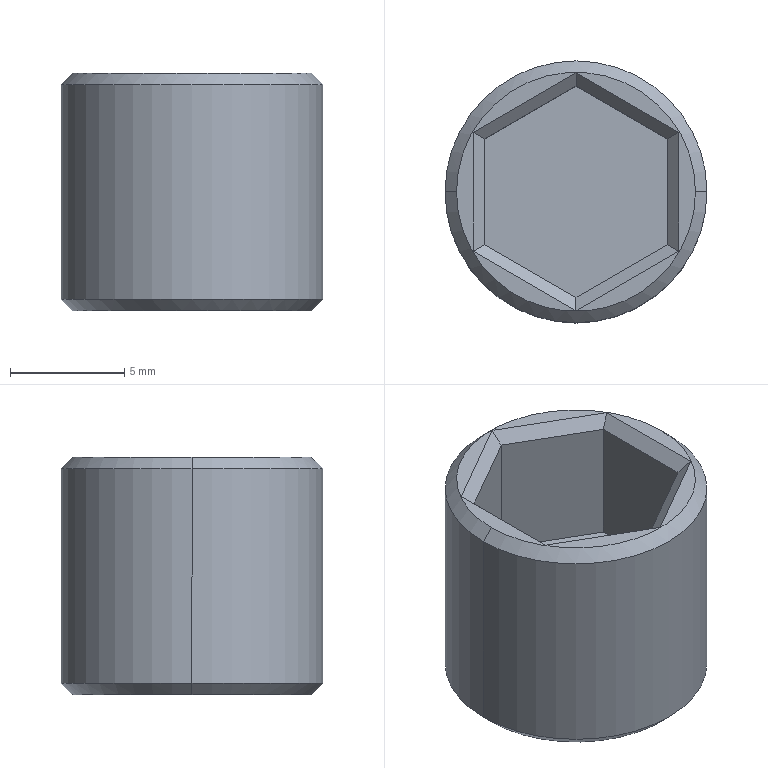Part | SolidWorks | features BaseBody 1 | 1 solid | 21 faces | box 11.45 x 11.45 x 10.4 mm | volume 725.97 mm3 | plane 15 | cone 4 | cylinder 2 | commonest cylinder face diameters 11.45 x2
STEP:
#1=CARTESIAN_POINT('',(5.725,0.,0.5));
#2=VERTEX_POINT('',#1);
#3=CARTESIAN_POINT('',(-5.725,0.,0.5));
#4=VERTEX_POINT('',#3);
#5=CARTESIAN_POINT('',(0.,0.,0.5));
#6=DIRECTION('',(0.,0.,1.));
#7=DIRECTION('',(1.,0.,0.));
#8=AXIS2_PLACEMENT_3D('',#5,#6,#7);
#9=CIRCLE('',#8,5.725);
#10=EDGE_CURVE('',#2,#4,#9,.T.);
#11=ORIENTED_EDGE('',*,*,#10,.T.);
#12=CARTESIAN_POINT('',(-5.725,0.,9.9));
#13=VERTEX_POINT('',#12);
#14=CARTESIAN_POINT('',(-5.725,0.,0.));
#15=DIRECTION('',(0.,0.,1.));
#16=VECTOR('',#15,1000.);
#17=LINE('',#14,#16);
#18=EDGE_CURVE('',#4,#13,#17,.T.);
#19=ORIENTED_EDGE('',*,*,#18,.T.);
#20=CARTESIAN_POINT('',(5.725,0.,9.9));
#21=VERTEX_POINT('',#20);
#22=CARTESIAN_POINT('',(0.,0.,9.9));
#23=DIRECTION('',(0.,0.,-1.));
#24=DIRECTION('',(1.,0.,0.));
#25=AXIS2_PLACEMENT_3D('',#22,#23,#24);
#26=CIRCLE('',#25,5.725);
#27=EDGE_CURVE('',#13,#21,#26,.T.);
#28=ORIENTED_EDGE('',*,*,#27,.T.);
#29=CARTESIAN_POINT('',(5.725,0.,0.));
#30=DIRECTION('',(0.,0.,1.));
#31=VECTOR('',#30,1000.);
#32=LINE('',#29,#31);
#33=EDGE_CURVE('',#2,#21,#32,.T.);
#34=ORIENTED_EDGE('',*,*,#33,.F.);
#35=EDGE_LOOP('',(#11,#19,#28,#34));
#36=FACE_OUTER_BOUND('',#35,.T.);
#37=CARTESIAN_POINT('',(0.,0.,0.));
#38=DIRECTION('',(0.,0.,1.));
#39=DIRECTION('',(1.,0.,0.));
#40=AXIS2_PLACEMENT_3D('',#37,#38,#39);
#41=CYLINDRICAL_SURFACE('',#40,5.725);
#42=ADVANCED_FACE('',(#36),#41,.T.);
#43=CARTESIAN_POINT('',(-5.225,0.,10.4));
#44=VERTEX_POINT('',#43);
#45=CARTESIAN_POINT('',(5.225,0.,10.4));
#46=VERTEX_POINT('',#45);
#47=CARTESIAN_POINT('',(0.,0.,10.4));
#48=DIRECTION('',(0.,0.,-1.));
#49=DIRECTION('',(-1.,0.,0.));
#50=AXIS2_PLACEMENT_3D('',#47,#48,#49);
#51=CIRCLE('',#50,5.225);
#52=EDGE_CURVE('',#44,#46,#51,.T.);
#53=ORIENTED_EDGE('',*,*,#52,.T.);
#54=CARTESIAN_POINT('',(5.725,0.,9.9));
#55=DIRECTION('',(0.7071,0.,-0.7071));
#56=VECTOR('',#55,1000.);
#57=LINE('',#54,#56);
#58=EDGE_CURVE('',#46,#21,#57,.T.);
#59=ORIENTED_EDGE('',*,*,#58,.T.);
#60=ORIENTED_EDGE('',*,*,#27,.F.);
#61=CARTESIAN_POINT('',(-5.725,0.,9.9));
#62=DIRECTION('',(-0.7071,0.,-0.7071));
#63=VECTOR('',#62,1000.);
#64=LINE('',#61,#63);
#65=EDGE_CURVE('',#44,#13,#64,.T.);
#66=ORIENTED_EDGE('',*,*,#65,.F.);
#67=EDGE_LOOP('',(#53,#59,#60,#66));
#68=FACE_OUTER_BOUND('',#67,.T.);
#69=CARTESIAN_POINT('',(0.,0.,9.9));
#70=DIRECTION('',(0.,0.,-1.));
#71=DIRECTION('',(-1.,0.,0.));
#72=AXIS2_PLACEMENT_3D('',#69,#70,#71);
#73=CONICAL_SURFACE('',#72,5.725,0.7854);
#74=ADVANCED_FACE('',(#68),#73,.T.);
#75=CARTESIAN_POINT('',(5.225,0.,0.));
#76=VERTEX_POINT('',#75);
#77=CARTESIAN_POINT('',(-5.225,0.,0.));
#78=VERTEX_POINT('',#77);
#79=CARTESIAN_POINT('',(0.,0.,0.));
#80=DIRECTION('',(0.,0.,1.));
#81=DIRECTION('',(1.,0.,0.));
#82=AXIS2_PLACEMENT_3D('',#79,#80,#81);
#83=CIRCLE('',#82,5.225);
#84=EDGE_CURVE('',#76,#78,#83,.T.);
#85=ORIENTED_EDGE('',*,*,#84,.T.);
#86=CARTESIAN_POINT('',(-5.725,0.,0.5));
#87=DIRECTION('',(-0.7071,0.,0.7071));
#88=VECTOR('',#87,1000.);
#89=LINE('',#86,#88);
#90=EDGE_CURVE('',#78,#4,#89,.T.);
#91=ORIENTED_EDGE('',*,*,#90,.T.);
#92=ORIENTED_EDGE('',*,*,#10,.F.);
#93=CARTESIAN_POINT('',(5.725,0.,0.5));
#94=DIRECTION('',(0.7071,0.,0.7071));
#95=VECTOR('',#94,1000.);
#96=LINE('',#93,#95);
#97=EDGE_CURVE('',#76,#2,#96,.T.);
#98=ORIENTED_EDGE('',*,*,#97,.F.);
#99=EDGE_LOOP('',(#85,#91,#92,#98));
#100=FACE_OUTER_BOUND('',#99,.T.);
#101=CARTESIAN_POINT('',(0.,0.,0.5));
#102=DIRECTION('',(0.,0.,1.));
#103=DIRECTION('',(1.,0.,0.));
#104=AXIS2_PLACEMENT_3D('',#101,#102,#103);
#105=CONICAL_SURFACE('',#104,5.725,0.7854);
#106=ADVANCED_FACE('',(#100),#105,.T.);
#107=ORIENTED_EDGE('',*,*,#18,.F.);
#108=CARTESIAN_POINT('',(0.,0.,0.5));
#109=DIRECTION('',(0.,0.,1.));
#110=DIRECTION('',(1.,0.,0.));
#111=AXIS2_PLACEMENT_3D('',#108,#109,#110);
#112=CIRCLE('',#111,5.725);
#113=EDGE_CURVE('',#4,#2,#112,.T.);
#114=ORIENTED_EDGE('',*,*,#113,.T.);
#115=ORIENTED_EDGE('',*,*,#33,.T.);
#116=CARTESIAN_POINT('',(0.,0.,9.9));
#117=DIRECTION('',(0.,0.,-1.));
#118=DIRECTION('',(1.,0.,0.));
#119=AXIS2_PLACEMENT_3D('',#116,#117,#118);
#120=CIRCLE('',#119,5.725);
#121=EDGE_CURVE('',#21,#13,#120,.T.);
#122=ORIENTED_EDGE('',*,*,#121,.T.);
#123=EDGE_LOOP('',(#107,#114,#115,#122));
#124=FACE_OUTER_BOUND('',#123,.T.);
#125=CARTESIAN_POINT('',(0.,0.,0.));
#126=DIRECTION('',(0.,0.,1.));
#127=DIRECTION('',(1.,0.,0.));
#128=AXIS2_PLACEMENT_3D('',#125,#126,#127);
#129=CYLINDRICAL_SURFACE('',#128,5.725);
#130=ADVANCED_FACE('',(#124),#129,.T.);
#131=ORIENTED_EDGE('',*,*,#58,.F.);
#132=CARTESIAN_POINT('',(0.,0.,10.4));
#133=DIRECTION('',(0.,0.,-1.));
#134=DIRECTION('',(-1.,0.,0.));
#135=AXIS2_PLACEMENT_3D('',#132,#133,#134);
#136=CIRCLE('',#135,5.225);
#137=EDGE_CURVE('',#46,#44,#136,.T.);
#138=ORIENTED_EDGE('',*,*,#137,.T.);
#139=ORIENTED_EDGE('',*,*,#65,.T.);
#140=ORIENTED_EDGE('',*,*,#121,.F.);
#141=EDGE_LOOP('',(#131,#138,#139,#140));
#142=FACE_OUTER_BOUND('',#141,.T.);
#143=CARTESIAN_POINT('',(0.,0.,9.9));
#144=DIRECTION('',(0.,0.,-1.));
#145=DIRECTION('',(-1.,0.,0.));
#146=AXIS2_PLACEMENT_3D('',#143,#144,#145);
#147=CONICAL_SURFACE('',#146,5.725,0.7854);
#148=ADVANCED_FACE('',(#142),#147,.T.);
#149=ORIENTED_EDGE('',*,*,#90,.F.);
#150=CARTESIAN_POINT('',(0.,0.,0.));
#151=DIRECTION('',(0.,0.,1.));
#152=DIRECTION('',(1.,0.,0.));
#153=AXIS2_PLACEMENT_3D('',#150,#151,#152);
#154=CIRCLE('',#153,5.225);
#155=EDGE_CURVE('',#78,#76,#154,.T.);
#156=ORIENTED_EDGE('',*,*,#155,.T.);
#157=ORIENTED_EDGE('',*,*,#97,.T.);
#158=ORIENTED_EDGE('',*,*,#113,.F.);
#159=EDGE_LOOP('',(#149,#156,#157,#158));
#160=FACE_OUTER_BOUND('',#159,.T.);
#161=CARTESIAN_POINT('',(0.,0.,0.5));
#162=DIRECTION('',(0.,0.,1.));
#163=DIRECTION('',(1.,0.,0.));
#164=AXIS2_PLACEMENT_3D('',#161,#162,#163);
#165=CONICAL_SURFACE('',#164,5.725,0.7854);
#166=ADVANCED_FACE('',(#160),#165,.T.);
#167=CARTESIAN_POINT('',(4.5,-2.598,10.4));
#168=VERTEX_POINT('',#167);
#169=CARTESIAN_POINT('',(4.5,2.598,10.4));
#170=VERTEX_POINT('',#169);
#171=CARTESIAN_POINT('',(4.5,0.,10.4));
#172=DIRECTION('',(0.,1.,0.));
#173=VECTOR('',#172,1000.);
#174=LINE('',#171,#173);
#175=EDGE_CURVE('',#168,#170,#174,.T.);
#176=ORIENTED_EDGE('',*,*,#175,.F.);
#177=CARTESIAN_POINT('',(0.,-5.196,10.4));
#178=VERTEX_POINT('',#177);
#179=CARTESIAN_POINT('',(0.,-5.196,10.4));
#180=DIRECTION('',(0.866,0.5,0.));
#181=VECTOR('',#180,1000.);
#182=LINE('',#179,#181);
#183=EDGE_CURVE('',#178,#168,#182,.T.);
#184=ORIENTED_EDGE('',*,*,#183,.F.);
#185=CARTESIAN_POINT('',(-4.5,-2.598,10.4));
#186=VERTEX_POINT('',#185);
#187=CARTESIAN_POINT('',(-4.5,-2.598,10.4));
#188=DIRECTION('',(0.866,-0.5,0.));
#189=VECTOR('',#188,1000.);
#190=LINE('',#187,#189);
#191=EDGE_CURVE('',#186,#178,#190,.T.);
#192=ORIENTED_EDGE('',*,*,#191,.F.);
#193=CARTESIAN_POINT('',(-4.5,2.598,10.4));
#194=VERTEX_POINT('',#193);
#195=CARTESIAN_POINT('',(-4.5,0.,10.4));
#196=DIRECTION('',(0.,-1.,0.));
#197=VECTOR('',#196,1000.);
#198=LINE('',#195,#197);
#199=EDGE_CURVE('',#194,#186,#198,.T.);
#200=ORIENTED_EDGE('',*,*,#199,.F.);
#201=CARTESIAN_POINT('',(0.,5.196,10.4));
#202=VERTEX_POINT('',#201);
#203=CARTESIAN_POINT('',(0.,5.196,10.4));
#204=DIRECTION('',(-0.866,-0.5,0.));
#205=VECTOR('',#204,1000.);
#206=LINE('',#203,#205);
#207=EDGE_CURVE('',#202,#194,#206,.T.);
#208=ORIENTED_EDGE('',*,*,#207,.F.);
#209=CARTESIAN_POINT('',(4.5,2.598,10.4));
#210=DIRECTION('',(-0.866,0.5,0.));
#211=VECTOR('',#210,1000.);
#212=LINE('',#209,#211);
#213=EDGE_CURVE('',#170,#202,#212,.T.);
#214=ORIENTED_EDGE('',*,*,#213,.F.);
#215=EDGE_LOOP('',(#176,#184,#192,#200,#208,#214));
#216=FACE_BOUND('',#215,.T.);
#217=ORIENTED_EDGE('',*,*,#52,.F.);
#218=ORIENTED_EDGE('',*,*,#137,.F.);
#219=EDGE_LOOP('',(#217,#218));
#220=FACE_OUTER_BOUND('',#219,.T.);
#221=CARTESIAN_POINT('',(0.,0.,10.4));
#222=DIRECTION('',(0.,0.,-1.));
#223=DIRECTION('',(-1.,0.,0.));
#224=AXIS2_PLACEMENT_3D('',#221,#222,#223);
#225=PLANE('',#224);
#226=ADVANCED_FACE('',(#216,#220),#225,.F.);
#227=ORIENTED_EDGE('',*,*,#84,.F.);
#228=ORIENTED_EDGE('',*,*,#155,.F.);
#229=EDGE_LOOP('',(#227,#228));
#230=FACE_OUTER_BOUND('',#229,.T.);
#231=CARTESIAN_POINT('',(0.,0.,0.));
#232=DIRECTION('',(0.,0.,-1.));
#233=DIRECTION('',(-1.,0.,0.));
#234=AXIS2_PLACEMENT_3D('',#231,#232,#233);
#235=PLANE('',#234);
#236=ADVANCED_FACE('',(#230),#235,.T.);
#237=CARTESIAN_POINT('',(0.,4.619,9.9));
#238=VERTEX_POINT('',#237);
#239=CARTESIAN_POINT('',(0.,3.876,9.257));
#240=DIRECTION('',(0.,-0.7559,-0.6547));
#241=VECTOR('',#240,1000.);
#242=LINE('',#239,#241);
#243=EDGE_CURVE('',#202,#238,#242,.T.);
#244=ORIENTED_EDGE('',*,*,#243,.T.);
#245=CARTESIAN_POINT('',(4.,2.309,9.9));
#246=VERTEX_POINT('',#245);
#247=CARTESIAN_POINT('',(0.,4.619,9.9));
#248=DIRECTION('',(0.866,-0.5,0.));
#249=VECTOR('',#248,1000.);
#250=LINE('',#247,#249);
#251=EDGE_CURVE('',#238,#246,#250,.T.);
#252=ORIENTED_EDGE('',*,*,#251,.T.);
#253=CARTESIAN_POINT('',(4.,2.309,9.9));
#254=DIRECTION('',(0.6547,0.378,0.6547));
#255=VECTOR('',#254,1000.);
#256=LINE('',#253,#255);
#257=EDGE_CURVE('',#246,#170,#256,.T.);
#258=ORIENTED_EDGE('',*,*,#257,.T.);
#259=ORIENTED_EDGE('',*,*,#213,.T.);
#260=EDGE_LOOP('',(#244,#252,#258,#259));
#261=FACE_OUTER_BOUND('',#260,.T.);
#262=CARTESIAN_POINT('',(3.125,3.103,10.15));
#263=DIRECTION('',(-0.3536,-0.6124,0.7071));
#264=DIRECTION('',(0.,-0.7559,-0.6547));
#265=AXIS2_PLACEMENT_3D('',#262,#263,#264);
#266=PLANE('',#265);
#267=ADVANCED_FACE('',(#261),#266,.T.);
#268=ORIENTED_EDGE('',*,*,#257,.F.);
#269=CARTESIAN_POINT('',(4.,-2.309,9.9));
#270=VERTEX_POINT('',#269);
#271=CARTESIAN_POINT('',(4.,-1.155,9.9));
#272=DIRECTION('',(0.,-1.,0.));
#273=VECTOR('',#272,1000.);
#274=LINE('',#271,#273);
#275=EDGE_CURVE('',#246,#270,#274,.T.);
#276=ORIENTED_EDGE('',*,*,#275,.T.);
#277=CARTESIAN_POINT('',(4.,-2.309,9.9));
#278=DIRECTION('',(0.6547,-0.378,0.6547));
#279=VECTOR('',#278,1000.);
#280=LINE('',#277,#279);
#281=EDGE_CURVE('',#270,#168,#280,.T.);
#282=ORIENTED_EDGE('',*,*,#281,.T.);
#283=ORIENTED_EDGE('',*,*,#175,.T.);
#284=EDGE_LOOP('',(#268,#276,#282,#283));
#285=FACE_OUTER_BOUND('',#284,.T.);
#286=CARTESIAN_POINT('',(4.25,-1.155,10.15));
#287=DIRECTION('',(-0.7071,0.,0.7071));
#288=DIRECTION('',(0.7071,0.,0.7071));
#289=AXIS2_PLACEMENT_3D('',#286,#287,#288);
#290=PLANE('',#289);
#291=ADVANCED_FACE('',(#285),#290,.T.);
#292=ORIENTED_EDGE('',*,*,#281,.F.);
#293=CARTESIAN_POINT('',(0.,-4.619,9.9));
#294=VERTEX_POINT('',#293);
#295=CARTESIAN_POINT('',(4.,-2.309,9.9));
#296=DIRECTION('',(-0.866,-0.5,0.));
#297=VECTOR('',#296,1000.);
#298=LINE('',#295,#297);
#299=EDGE_CURVE('',#270,#294,#298,.T.);
#300=ORIENTED_EDGE('',*,*,#299,.T.);
#301=CARTESIAN_POINT('',(0.,-4.536,9.829));
#302=DIRECTION('',(0.,-0.7559,0.6547));
#303=VECTOR('',#302,1000.);
#304=LINE('',#301,#303);
#305=EDGE_CURVE('',#294,#178,#304,.T.);
#306=ORIENTED_EDGE('',*,*,#305,.T.);
#307=ORIENTED_EDGE('',*,*,#183,.T.);
#308=EDGE_LOOP('',(#292,#300,#306,#307));
#309=FACE_OUTER_BOUND('',#308,.T.);
#310=CARTESIAN_POINT('',(1.125,-4.258,10.15));
#311=DIRECTION('',(-0.3536,0.6124,0.7071));
#312=DIRECTION('',(0.,-0.7559,0.6547));
#313=AXIS2_PLACEMENT_3D('',#310,#311,#312);
#314=PLANE('',#313);
#315=ADVANCED_FACE('',(#309),#314,.T.);
#316=ORIENTED_EDGE('',*,*,#305,.F.);
#317=CARTESIAN_POINT('',(-4.,-2.309,9.9));
#318=VERTEX_POINT('',#317);
#319=CARTESIAN_POINT('',(0.,-4.619,9.9));
#320=DIRECTION('',(-0.866,0.5,0.));
#321=VECTOR('',#320,1000.);
#322=LINE('',#319,#321);
#323=EDGE_CURVE('',#294,#318,#322,.T.);
#324=ORIENTED_EDGE('',*,*,#323,.T.);
#325=CARTESIAN_POINT('',(-4.,-2.309,9.9));
#326=DIRECTION('',(-0.6547,-0.378,0.6547));
#327=VECTOR('',#326,1000.);
#328=LINE('',#325,#327);
#329=EDGE_CURVE('',#318,#186,#328,.T.);
#330=ORIENTED_EDGE('',*,*,#329,.T.);
#331=ORIENTED_EDGE('',*,*,#191,.T.);
#332=EDGE_LOOP('',(#316,#324,#330,#331));
#333=FACE_OUTER_BOUND('',#332,.T.);
#334=CARTESIAN_POINT('',(-3.125,-3.103,10.15));
#335=DIRECTION('',(0.3536,0.6124,0.7071));
#336=DIRECTION('',(0.,-0.7559,0.6547));
#337=AXIS2_PLACEMENT_3D('',#334,#335,#336);
#338=PLANE('',#337);
#339=ADVANCED_FACE('',(#333),#338,.T.);
#340=ORIENTED_EDGE('',*,*,#329,.F.);
#341=CARTESIAN_POINT('',(-4.,2.309,9.9));
#342=VERTEX_POINT('',#341);
#343=CARTESIAN_POINT('',(-4.,1.155,9.9));
#344=DIRECTION('',(0.,1.,0.));
#345=VECTOR('',#344,1000.);
#346=LINE('',#343,#345);
#347=EDGE_CURVE('',#318,#342,#346,.T.);
#348=ORIENTED_EDGE('',*,*,#347,.T.);
#349=CARTESIAN_POINT('',(-4.,2.309,9.9));
#350=DIRECTION('',(-0.6547,0.378,0.6547));
#351=VECTOR('',#350,1000.);
#352=LINE('',#349,#351);
#353=EDGE_CURVE('',#342,#194,#352,.T.);
#354=ORIENTED_EDGE('',*,*,#353,.T.);
#355=ORIENTED_EDGE('',*,*,#199,.T.);
#356=EDGE_LOOP('',(#340,#348,#354,#355));
#357=FACE_OUTER_BOUND('',#356,.T.);
#358=CARTESIAN_POINT('',(-4.25,1.155,10.15));
#359=DIRECTION('',(0.7071,0.,0.7071));
#360=DIRECTION('',(0.7071,0.,-0.7071));
#361=AXIS2_PLACEMENT_3D('',#358,#359,#360);
#362=PLANE('',#361);
#363=ADVANCED_FACE('',(#357),#362,.T.);
#364=ORIENTED_EDGE('',*,*,#353,.F.);
#365=CARTESIAN_POINT('',(-4.,2.309,9.9));
#366=DIRECTION('',(0.866,0.5,0.));
#367=VECTOR('',#366,1000.);
#368=LINE('',#365,#367);
#369=EDGE_CURVE('',#342,#238,#368,.T.);
#370=ORIENTED_EDGE('',*,*,#369,.T.);
#371=ORIENTED_EDGE('',*,*,#243,.F.);
#372=ORIENTED_EDGE('',*,*,#207,.T.);
#373=EDGE_LOOP('',(#364,#370,#371,#372));
#374=FACE_OUTER_BOUND('',#373,.T.);
#375=CARTESIAN_POINT('',(-1.125,4.258,10.15));
#376=DIRECTION('',(0.3536,-0.6124,0.7071));
#377=DIRECTION('',(0.,-0.7559,-0.6547));
#378=AXIS2_PLACEMENT_3D('',#375,#376,#377);
#379=PLANE('',#378);
#380=ADVANCED_FACE('',(#374),#379,.T.);
#381=CARTESIAN_POINT('',(4.,2.309,4.4));
#382=VERTEX_POINT('',#381);
#383=CARTESIAN_POINT('',(0.,4.619,4.4));
#384=VERTEX_POINT('',#383);
#385=CARTESIAN_POINT('',(4.,2.309,4.4));
#386=DIRECTION('',(-0.866,0.5,0.));
#387=VECTOR('',#386,1000.);
#388=LINE('',#385,#387);
#389=EDGE_CURVE('',#382,#384,#388,.T.);
#390=ORIENTED_EDGE('',*,*,#389,.F.);
#391=CARTESIAN_POINT('',(4.,2.309,10.4));
#392=DIRECTION('',(0.,0.,-1.));
#393=VECTOR('',#392,1000.);
#394=LINE('',#391,#393);
#395=EDGE_CURVE('',#246,#382,#394,.T.);
#396=ORIENTED_EDGE('',*,*,#395,.F.);
#397=ORIENTED_EDGE('',*,*,#251,.F.);
#398=CARTESIAN_POINT('',(0.,4.619,10.4));
#399=DIRECTION('',(0.,0.,1.));
#400=VECTOR('',#399,1000.);
#401=LINE('',#398,#400);
#402=EDGE_CURVE('',#384,#238,#401,.T.);
#403=ORIENTED_EDGE('',*,*,#402,.F.);
#404=EDGE_LOOP('',(#390,#396,#397,#403));
#405=FACE_OUTER_BOUND('',#404,.T.);
#406=CARTESIAN_POINT('',(4.,2.309,10.4));
#407=DIRECTION('',(0.5,0.866,0.));
#408=DIRECTION('',(-0.866,0.5,0.));
#409=AXIS2_PLACEMENT_3D('',#406,#407,#408);
#410=PLANE('',#409);
#411=ADVANCED_FACE('',(#405),#410,.F.);
#412=CARTESIAN_POINT('',(4.,-2.309,4.4));
#413=VERTEX_POINT('',#412);
#414=CARTESIAN_POINT('',(4.,-2.309,4.4));
#415=DIRECTION('',(0.,1.,0.));
#416=VECTOR('',#415,1000.);
#417=LINE('',#414,#416);
#418=EDGE_CURVE('',#413,#382,#417,.T.);
#419=ORIENTED_EDGE('',*,*,#418,.F.);
#420=CARTESIAN_POINT('',(4.,-2.309,10.4));
#421=DIRECTION('',(0.,0.,-1.));
#422=VECTOR('',#421,1000.);
#423=LINE('',#420,#422);
#424=EDGE_CURVE('',#270,#413,#423,.T.);
#425=ORIENTED_EDGE('',*,*,#424,.F.);
#426=ORIENTED_EDGE('',*,*,#275,.F.);
#427=ORIENTED_EDGE('',*,*,#395,.T.);
#428=EDGE_LOOP('',(#419,#425,#426,#427));
#429=FACE_OUTER_BOUND('',#428,.T.);
#430=CARTESIAN_POINT('',(4.,-2.309,10.4));
#431=DIRECTION('',(1.,0.,0.));
#432=DIRECTION('',(0.,0.,-1.));
#433=AXIS2_PLACEMENT_3D('',#430,#431,#432);
#434=PLANE('',#433);
#435=ADVANCED_FACE('',(#429),#434,.F.);
#436=CARTESIAN_POINT('',(0.,-4.619,4.4));
#437=VERTEX_POINT('',#436);
#438=CARTESIAN_POINT('',(0.,-4.619,4.4));
#439=DIRECTION('',(0.866,0.5,0.));
#440=VECTOR('',#439,1000.);
#441=LINE('',#438,#440);
#442=EDGE_CURVE('',#437,#413,#441,.T.);
#443=ORIENTED_EDGE('',*,*,#442,.F.);
#444=CARTESIAN_POINT('',(0.,-4.619,10.4));
#445=DIRECTION('',(0.,0.,-1.));
#446=VECTOR('',#445,1000.);
#447=LINE('',#444,#446);
#448=EDGE_CURVE('',#294,#437,#447,.T.);
#449=ORIENTED_EDGE('',*,*,#448,.F.);
#450=ORIENTED_EDGE('',*,*,#299,.F.);
#451=ORIENTED_EDGE('',*,*,#424,.T.);
#452=EDGE_LOOP('',(#443,#449,#450,#451));
#453=FACE_OUTER_BOUND('',#452,.T.);
#454=CARTESIAN_POINT('',(0.,-4.619,10.4));
#455=DIRECTION('',(0.5,-0.866,0.));
#456=DIRECTION('',(0.866,0.5,0.));
#457=AXIS2_PLACEMENT_3D('',#454,#455,#456);
#458=PLANE('',#457);
#459=ADVANCED_FACE('',(#453),#458,.F.);
#460=CARTESIAN_POINT('',(-4.,-2.309,4.4));
#461=VERTEX_POINT('',#460);
#462=CARTESIAN_POINT('',(-4.,-2.309,4.4));
#463=DIRECTION('',(0.866,-0.5,0.));
#464=VECTOR('',#463,1000.);
#465=LINE('',#462,#464);
#466=EDGE_CURVE('',#461,#437,#465,.T.);
#467=ORIENTED_EDGE('',*,*,#466,.F.);
#468=CARTESIAN_POINT('',(-4.,-2.309,10.4));
#469=DIRECTION('',(0.,0.,-1.));
#470=VECTOR('',#469,1000.);
#471=LINE('',#468,#470);
#472=EDGE_CURVE('',#318,#461,#471,.T.);
#473=ORIENTED_EDGE('',*,*,#472,.F.);
#474=ORIENTED_EDGE('',*,*,#323,.F.);
#475=ORIENTED_EDGE('',*,*,#448,.T.);
#476=EDGE_LOOP('',(#467,#473,#474,#475));
#477=FACE_OUTER_BOUND('',#476,.T.);
#478=CARTESIAN_POINT('',(-4.,-2.309,10.4));
#479=DIRECTION('',(-0.5,-0.866,0.));
#480=DIRECTION('',(0.866,-0.5,0.));
#481=AXIS2_PLACEMENT_3D('',#478,#479,#480);
#482=PLANE('',#481);
#483=ADVANCED_FACE('',(#477),#482,.F.);
#484=CARTESIAN_POINT('',(-4.,2.309,4.4));
#485=VERTEX_POINT('',#484);
#486=CARTESIAN_POINT('',(-4.,2.309,4.4));
#487=DIRECTION('',(0.,-1.,0.));
#488=VECTOR('',#487,1000.);
#489=LINE('',#486,#488);
#490=EDGE_CURVE('',#485,#461,#489,.T.);
#491=ORIENTED_EDGE('',*,*,#490,.F.);
#492=CARTESIAN_POINT('',(-4.,2.309,10.4));
#493=DIRECTION('',(0.,0.,-1.));
#494=VECTOR('',#493,1000.);
#495=LINE('',#492,#494);
#496=EDGE_CURVE('',#342,#485,#495,.T.);
#497=ORIENTED_EDGE('',*,*,#496,.F.);
#498=ORIENTED_EDGE('',*,*,#347,.F.);
#499=ORIENTED_EDGE('',*,*,#472,.T.);
#500=EDGE_LOOP('',(#491,#497,#498,#499));
#501=FACE_OUTER_BOUND('',#500,.T.);
#502=CARTESIAN_POINT('',(-4.,2.309,10.4));
#503=DIRECTION('',(-1.,0.,0.));
#504=DIRECTION('',(0.,0.,1.));
#505=AXIS2_PLACEMENT_3D('',#502,#503,#504);
#506=PLANE('',#505);
#507=ADVANCED_FACE('',(#501),#506,.F.);
#508=CARTESIAN_POINT('',(0.,4.619,4.4));
#509=DIRECTION('',(-0.866,-0.5,0.));
#510=VECTOR('',#509,1000.);
#511=LINE('',#508,#510);
#512=EDGE_CURVE('',#384,#485,#511,.T.);
#513=ORIENTED_EDGE('',*,*,#512,.F.);
#514=ORIENTED_EDGE('',*,*,#402,.T.);
#515=ORIENTED_EDGE('',*,*,#369,.F.);
#516=ORIENTED_EDGE('',*,*,#496,.T.);
#517=EDGE_LOOP('',(#513,#514,#515,#516));
#518=FACE_OUTER_BOUND('',#517,.T.);
#519=CARTESIAN_POINT('',(0.,4.619,10.4));
#520=DIRECTION('',(-0.5,0.866,0.));
#521=DIRECTION('',(-0.866,-0.5,0.));
#522=AXIS2_PLACEMENT_3D('',#519,#520,#521);
#523=PLANE('',#522);
#524=ADVANCED_FACE('',(#518),#523,.F.);
#525=ORIENTED_EDGE('',*,*,#389,.T.);
#526=ORIENTED_EDGE('',*,*,#512,.T.);
#527=ORIENTED_EDGE('',*,*,#490,.T.);
#528=ORIENTED_EDGE('',*,*,#466,.T.);
#529=ORIENTED_EDGE('',*,*,#442,.T.);
#530=ORIENTED_EDGE('',*,*,#418,.T.);
#531=EDGE_LOOP('',(#525,#526,#527,#528,#529,#530));
#532=FACE_OUTER_BOUND('',#531,.T.);
#533=CARTESIAN_POINT('',(0.,0.,4.4));
#534=DIRECTION('',(0.,0.,1.));
#535=DIRECTION('',(1.,0.,0.));
#536=AXIS2_PLACEMENT_3D('',#533,#534,#535);
#537=PLANE('',#536);
#538=ADVANCED_FACE('',(#532),#537,.T.);
#539=CLOSED_SHELL('',(#42,#74,#106,#130,#148,#166,#226,#236,#267,#291,#315,#339,#363,#380,#411,#435,#459,#483,#507,#524,#538));
#540=MANIFOLD_SOLID_BREP('',#539);
#541=CARTESIAN_POINT('',(0.,0.,0.));
#542=DIRECTION('',(0.,0.,1.));
#543=DIRECTION('',(1.,0.,0.));
#544=AXIS2_PLACEMENT_3D('',#541,#542,#543);
#545=(LENGTH_UNIT()NAMED_UNIT(*)SI_UNIT(.MILLI.,.METRE.));
#546=UNCERTAINTY_MEASURE_WITH_UNIT(LENGTH_MEASURE(0.00001),#545,'','');
#547=(NAMED_UNIT(*)PLANE_ANGLE_UNIT()SI_UNIT($,.RADIAN.));
#548=(NAMED_UNIT(*)SI_UNIT($,.STERADIAN.)SOLID_ANGLE_UNIT());
#549=(GEOMETRIC_REPRESENTATION_CONTEXT(3)GLOBAL_UNCERTAINTY_ASSIGNED_CONTEXT((#546))GLOBAL_UNIT_ASSIGNED_CONTEXT((#545,#547,#548))REPRESENTATION_CONTEXT('',''));
#550=ADVANCED_BREP_SHAPE_REPRESENTATION('',(#540,#544),#549);